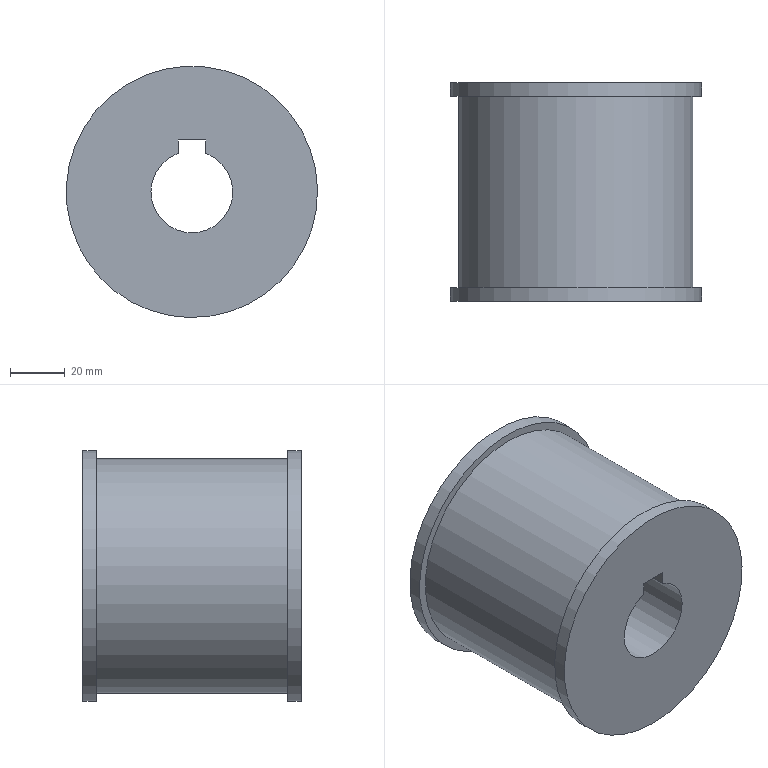Part | STEP file | SN10_001_009_POLIA | 1 solid | 11 faces | box 92 x 80 x 92 mm | volume 413118 mm3 | plane 7 | cylinder 4 | commonest cylinder face diameters 92 x2 30 x1 86 x1
STEP:
#1=CARTESIAN_POINT('',(0.,0.,0.));
#2=DIRECTION('',(0.,0.,1.));
#3=DIRECTION('',(1.,0.,0.));
#4=AXIS2_PLACEMENT_3D('',#1,#2,#3);
#5=CARTESIAN_POINT('',(6005.,-140.,19.));
#6=VERTEX_POINT('',#5);
#7=CARTESIAN_POINT('',(5995.,-140.,19.));
#8=VERTEX_POINT('',#7);
#9=CARTESIAN_POINT('',(6005.,-140.,19.));
#10=DIRECTION('',(-1.,0.,0.));
#11=VECTOR('',#10,1.);
#12=LINE('',#9,#11);
#13=CARTESIAN_POINT('',(6005.,-60.,19.));
#14=DIRECTION('',(0.,0.,1.));
#15=DIRECTION('',(1.,0.,0.));
#16=AXIS2_PLACEMENT_3D('',#13,#14,#15);
#17=PLANE('',#16);
#18=CARTESIAN_POINT('',(0.,-80.));
#19=DIRECTION('',(-1.,0.));
#20=VECTOR('',#19,1.);
#21=LINE('',#18,#20);
#22=(GEOMETRIC_REPRESENTATION_CONTEXT(2)PARAMETRIC_REPRESENTATION_CONTEXT()REPRESENTATION_CONTEXT('',''));
#23=DEFINITIONAL_REPRESENTATION('',(#21),#22);
#24=PCURVE('',#17,#23);
#25=CARTESIAN_POINT('',(6000.,-140.,0.));
#26=DIRECTION('',(0.,1.,0.));
#27=DIRECTION('',(0.,0.,1.));
#28=AXIS2_PLACEMENT_3D('',#25,#26,#27);
#29=PLANE('',#28);
#30=CARTESIAN_POINT('',(19.,5.));
#31=DIRECTION('',(0.,-1.));
#32=VECTOR('',#31,1.);
#33=LINE('',#30,#32);
#34=(GEOMETRIC_REPRESENTATION_CONTEXT(2)PARAMETRIC_REPRESENTATION_CONTEXT()REPRESENTATION_CONTEXT('',''));
#35=DEFINITIONAL_REPRESENTATION('',(#33),#34);
#36=PCURVE('',#29,#35);
#37=SURFACE_CURVE('',#12,(#24,#36),.PCURVE_S1.);
#38=EDGE_CURVE('',#6,#8,#37,.T.);
#39=ORIENTED_EDGE('',*,*,#38,.T.);
#40=CARTESIAN_POINT('',(5995.,-60.,19.));
#41=VERTEX_POINT('',#40);
#42=CARTESIAN_POINT('',(5995.,-60.,19.));
#43=DIRECTION('',(0.,-1.,0.));
#44=VECTOR('',#43,1.);
#45=LINE('',#42,#44);
#46=CARTESIAN_POINT('',(-10.,0.));
#47=DIRECTION('',(0.,-1.));
#48=VECTOR('',#47,1.);
#49=LINE('',#46,#48);
#50=(GEOMETRIC_REPRESENTATION_CONTEXT(2)PARAMETRIC_REPRESENTATION_CONTEXT()REPRESENTATION_CONTEXT('',''));
#51=DEFINITIONAL_REPRESENTATION('',(#49),#50);
#52=PCURVE('',#17,#51);
#53=CARTESIAN_POINT('',(5995.,-60.,11.));
#54=DIRECTION('',(1.,0.,0.));
#55=DIRECTION('',(0.,0.,-1.));
#56=AXIS2_PLACEMENT_3D('',#53,#54,#55);
#57=PLANE('',#56);
#58=CARTESIAN_POINT('',(-8.,0.));
#59=DIRECTION('',(0.,-1.));
#60=VECTOR('',#59,1.);
#61=LINE('',#58,#60);
#62=(GEOMETRIC_REPRESENTATION_CONTEXT(2)PARAMETRIC_REPRESENTATION_CONTEXT()REPRESENTATION_CONTEXT('',''));
#63=DEFINITIONAL_REPRESENTATION('',(#61),#62);
#64=PCURVE('',#57,#63);
#65=SURFACE_CURVE('',#45,(#52,#64),.PCURVE_S1.);
#66=EDGE_CURVE('',#41,#8,#65,.T.);
#67=ORIENTED_EDGE('',*,*,#66,.F.);
#68=CARTESIAN_POINT('',(6005.,-60.,19.));
#69=VERTEX_POINT('',#68);
#70=CARTESIAN_POINT('',(6005.,-60.,19.));
#71=DIRECTION('',(-1.,0.,0.));
#72=VECTOR('',#71,1.);
#73=LINE('',#70,#72);
#74=CARTESIAN_POINT('',(0.,0.));
#75=DIRECTION('',(-1.,0.));
#76=VECTOR('',#75,1.);
#77=LINE('',#74,#76);
#78=(GEOMETRIC_REPRESENTATION_CONTEXT(2)PARAMETRIC_REPRESENTATION_CONTEXT()REPRESENTATION_CONTEXT('',''));
#79=DEFINITIONAL_REPRESENTATION('',(#77),#78);
#80=PCURVE('',#17,#79);
#81=CARTESIAN_POINT('',(6000.,-60.,46.));
#82=DIRECTION('',(0.,1.,0.));
#83=DIRECTION('',(0.,0.,1.));
#84=AXIS2_PLACEMENT_3D('',#81,#82,#83);
#85=PLANE('',#84);
#86=CARTESIAN_POINT('',(-27.,5.));
#87=DIRECTION('',(0.,-1.));
#88=VECTOR('',#87,1.);
#89=LINE('',#86,#88);
#90=(GEOMETRIC_REPRESENTATION_CONTEXT(2)PARAMETRIC_REPRESENTATION_CONTEXT()REPRESENTATION_CONTEXT('',''));
#91=DEFINITIONAL_REPRESENTATION('',(#89),#90);
#92=PCURVE('',#85,#91);
#93=SURFACE_CURVE('',#73,(#80,#92),.PCURVE_S1.);
#94=EDGE_CURVE('',#69,#41,#93,.T.);
#95=ORIENTED_EDGE('',*,*,#94,.F.);
#96=CARTESIAN_POINT('',(6005.,-60.,19.));
#97=DIRECTION('',(0.,-1.,0.));
#98=VECTOR('',#97,1.);
#99=LINE('',#96,#98);
#100=CARTESIAN_POINT('',(0.,0.));
#101=DIRECTION('',(0.,-1.));
#102=VECTOR('',#101,1.);
#103=LINE('',#100,#102);
#104=(GEOMETRIC_REPRESENTATION_CONTEXT(2)PARAMETRIC_REPRESENTATION_CONTEXT()REPRESENTATION_CONTEXT('',''));
#105=DEFINITIONAL_REPRESENTATION('',(#103),#104);
#106=PCURVE('',#17,#105);
#107=CARTESIAN_POINT('',(6005.,-60.,19.));
#108=DIRECTION('',(-1.,0.,0.));
#109=DIRECTION('',(0.,0.,1.));
#110=AXIS2_PLACEMENT_3D('',#107,#108,#109);
#111=PLANE('',#110);
#112=CARTESIAN_POINT('',(0.,0.));
#113=DIRECTION('',(0.,-1.));
#114=VECTOR('',#113,1.);
#115=LINE('',#112,#114);
#116=(GEOMETRIC_REPRESENTATION_CONTEXT(2)PARAMETRIC_REPRESENTATION_CONTEXT()REPRESENTATION_CONTEXT('',''));
#117=DEFINITIONAL_REPRESENTATION('',(#115),#116);
#118=PCURVE('',#111,#117);
#119=SURFACE_CURVE('',#99,(#106,#118),.PCURVE_S1.);
#120=EDGE_CURVE('',#69,#6,#119,.T.);
#121=ORIENTED_EDGE('',*,*,#120,.T.);
#122=EDGE_LOOP('',(#39,#67,#95,#121));
#123=FACE_BOUND('',#122,.T.);
#124=ADVANCED_FACE('',(#123),#17,.F.);
#125=ORIENTED_EDGE('',*,*,#120,.F.);
#126=CARTESIAN_POINT('',(6005.,-60.,14.142));
#127=VERTEX_POINT('',#126);
#128=CARTESIAN_POINT('',(6005.,-60.,19.));
#129=DIRECTION('',(0.,0.,-1.));
#130=VECTOR('',#129,1.);
#131=LINE('',#128,#130);
#132=CARTESIAN_POINT('',(0.,0.));
#133=DIRECTION('',(-1.,0.));
#134=VECTOR('',#133,1.);
#135=LINE('',#132,#134);
#136=(GEOMETRIC_REPRESENTATION_CONTEXT(2)PARAMETRIC_REPRESENTATION_CONTEXT()REPRESENTATION_CONTEXT('',''));
#137=DEFINITIONAL_REPRESENTATION('',(#135),#136);
#138=PCURVE('',#111,#137);
#139=CARTESIAN_POINT('',(-27.,5.));
#140=DIRECTION('',(-1.,0.));
#141=VECTOR('',#140,1.);
#142=LINE('',#139,#141);
#143=(GEOMETRIC_REPRESENTATION_CONTEXT(2)PARAMETRIC_REPRESENTATION_CONTEXT()REPRESENTATION_CONTEXT('',''));
#144=DEFINITIONAL_REPRESENTATION('',(#142),#143);
#145=PCURVE('',#85,#144);
#146=SURFACE_CURVE('',#131,(#138,#145),.PCURVE_S1.);
#147=EDGE_CURVE('',#69,#127,#146,.T.);
#148=ORIENTED_EDGE('',*,*,#147,.T.);
#149=CARTESIAN_POINT('',(6005.,-140.,14.142));
#150=VERTEX_POINT('',#149);
#151=CARTESIAN_POINT('',(6005.,-60.,14.142));
#152=DIRECTION('',(0.,-1.,0.));
#153=VECTOR('',#152,1.);
#154=LINE('',#151,#153);
#155=CARTESIAN_POINT('',(-4.858,0.));
#156=DIRECTION('',(0.,-1.));
#157=VECTOR('',#156,1.);
#158=LINE('',#155,#157);
#159=(GEOMETRIC_REPRESENTATION_CONTEXT(2)PARAMETRIC_REPRESENTATION_CONTEXT()REPRESENTATION_CONTEXT('',''));
#160=DEFINITIONAL_REPRESENTATION('',(#158),#159);
#161=PCURVE('',#111,#160);
#162=CARTESIAN_POINT('',(6000.,-60.1,0.));
#163=DIRECTION('',(0.,-1.,0.));
#164=DIRECTION('',(0.8776,0.,0.4794));
#165=AXIS2_PLACEMENT_3D('',#162,#163,#164);
#166=CYLINDRICAL_SURFACE('',#165,15.);
#167=CARTESIAN_POINT('',(7.014,-0.1));
#168=DIRECTION('',(0.,1.));
#169=VECTOR('',#168,1.);
#170=LINE('',#167,#169);
#171=(GEOMETRIC_REPRESENTATION_CONTEXT(2)PARAMETRIC_REPRESENTATION_CONTEXT()REPRESENTATION_CONTEXT('',''));
#172=DEFINITIONAL_REPRESENTATION('',(#170),#171);
#173=PCURVE('',#166,#172);
#174=SURFACE_CURVE('',#154,(#161,#173),.PCURVE_S1.);
#175=EDGE_CURVE('',#127,#150,#174,.T.);
#176=ORIENTED_EDGE('',*,*,#175,.T.);
#177=CARTESIAN_POINT('',(6005.,-140.,19.));
#178=DIRECTION('',(0.,0.,-1.));
#179=VECTOR('',#178,1.);
#180=LINE('',#177,#179);
#181=CARTESIAN_POINT('',(0.,-80.));
#182=DIRECTION('',(-1.,0.));
#183=VECTOR('',#182,1.);
#184=LINE('',#181,#183);
#185=(GEOMETRIC_REPRESENTATION_CONTEXT(2)PARAMETRIC_REPRESENTATION_CONTEXT()REPRESENTATION_CONTEXT('',''));
#186=DEFINITIONAL_REPRESENTATION('',(#184),#185);
#187=PCURVE('',#111,#186);
#188=CARTESIAN_POINT('',(19.,5.));
#189=DIRECTION('',(-1.,0.));
#190=VECTOR('',#189,1.);
#191=LINE('',#188,#190);
#192=(GEOMETRIC_REPRESENTATION_CONTEXT(2)PARAMETRIC_REPRESENTATION_CONTEXT()REPRESENTATION_CONTEXT('',''));
#193=DEFINITIONAL_REPRESENTATION('',(#191),#192);
#194=PCURVE('',#29,#193);
#195=SURFACE_CURVE('',#180,(#187,#194),.PCURVE_S1.);
#196=EDGE_CURVE('',#6,#150,#195,.T.);
#197=ORIENTED_EDGE('',*,*,#196,.F.);
#198=EDGE_LOOP('',(#125,#148,#176,#197));
#199=FACE_BOUND('',#198,.T.);
#200=ADVANCED_FACE('',(#199),#111,.T.);
#201=CARTESIAN_POINT('',(5977.946,-60.,-40.369));
#202=VERTEX_POINT('',#201);
#203=CARTESIAN_POINT('',(6000.,-60.,0.));
#204=DIRECTION('',(0.,1.,0.));
#205=DIRECTION('',(1.,0.,0.));
#206=AXIS2_PLACEMENT_3D('',#203,#204,#205);
#207=CIRCLE('',#206,46.);
#208=CARTESIAN_POINT('',(-46.,0.));
#209=DIRECTION('',(0.,1.));
#210=AXIS2_PLACEMENT_2D('',#208,#209);
#211=CIRCLE('',#210,46.);
#212=(GEOMETRIC_REPRESENTATION_CONTEXT(2)PARAMETRIC_REPRESENTATION_CONTEXT()REPRESENTATION_CONTEXT('',''));
#213=DEFINITIONAL_REPRESENTATION('',(#211),#212);
#214=PCURVE('',#85,#213);
#215=CARTESIAN_POINT('',(6000.,-100.,0.));
#216=DIRECTION('',(0.,1.,0.));
#217=DIRECTION('',(0.4794,0.,0.8776));
#218=AXIS2_PLACEMENT_3D('',#215,#216,#217);
#219=CYLINDRICAL_SURFACE('',#218,46.);
#220=CARTESIAN_POINT('',(1.071,40.));
#221=DIRECTION('',(1.,0.));
#222=VECTOR('',#221,1.);
#223=LINE('',#220,#222);
#224=(GEOMETRIC_REPRESENTATION_CONTEXT(2)PARAMETRIC_REPRESENTATION_CONTEXT()REPRESENTATION_CONTEXT('',''));
#225=DEFINITIONAL_REPRESENTATION('',(#223),#224);
#226=PCURVE('',#219,#225);
#227=SURFACE_CURVE('',#207,(#214,#226),.PCURVE_S1.);
#228=EDGE_CURVE('',#202,#202,#227,.T.);
#229=ORIENTED_EDGE('',*,*,#228,.T.);
#230=EDGE_LOOP('',(#229));
#231=FACE_BOUND('',#230,.T.);
#232=CARTESIAN_POINT('',(5995.,-60.,14.142));
#233=VERTEX_POINT('',#232);
#234=CARTESIAN_POINT('',(6000.,-60.,0.));
#235=DIRECTION('',(0.,1.,0.));
#236=DIRECTION('',(1.,0.,0.));
#237=AXIS2_PLACEMENT_3D('',#234,#235,#236);
#238=CIRCLE('',#237,15.);
#239=CARTESIAN_POINT('',(-46.,0.));
#240=DIRECTION('',(0.,1.));
#241=AXIS2_PLACEMENT_2D('',#239,#240);
#242=CIRCLE('',#241,15.);
#243=(GEOMETRIC_REPRESENTATION_CONTEXT(2)PARAMETRIC_REPRESENTATION_CONTEXT()REPRESENTATION_CONTEXT('',''));
#244=DEFINITIONAL_REPRESENTATION('',(#242),#243);
#245=PCURVE('',#85,#244);
#246=CARTESIAN_POINT('',(12.066,-0.1));
#247=DIRECTION('',(-1.,0.));
#248=VECTOR('',#247,1.);
#249=LINE('',#246,#248);
#250=(GEOMETRIC_REPRESENTATION_CONTEXT(2)PARAMETRIC_REPRESENTATION_CONTEXT()REPRESENTATION_CONTEXT('',''));
#251=DEFINITIONAL_REPRESENTATION('',(#249),#250);
#252=PCURVE('',#166,#251);
#253=SURFACE_CURVE('',#238,(#245,#252),.PCURVE_S1.);
#254=EDGE_CURVE('',#127,#233,#253,.T.);
#255=ORIENTED_EDGE('',*,*,#254,.F.);
#256=ORIENTED_EDGE('',*,*,#147,.F.);
#257=ORIENTED_EDGE('',*,*,#94,.T.);
#258=CARTESIAN_POINT('',(5995.,-60.,14.142));
#259=DIRECTION('',(0.,0.,1.));
#260=VECTOR('',#259,1.);
#261=LINE('',#258,#260);
#262=CARTESIAN_POINT('',(-31.858,-5.));
#263=DIRECTION('',(1.,0.));
#264=VECTOR('',#263,1.);
#265=LINE('',#262,#264);
#266=(GEOMETRIC_REPRESENTATION_CONTEXT(2)PARAMETRIC_REPRESENTATION_CONTEXT()REPRESENTATION_CONTEXT('',''));
#267=DEFINITIONAL_REPRESENTATION('',(#265),#266);
#268=PCURVE('',#85,#267);
#269=CARTESIAN_POINT('',(-3.142,0.));
#270=DIRECTION('',(-1.,0.));
#271=VECTOR('',#270,1.);
#272=LINE('',#269,#271);
#273=(GEOMETRIC_REPRESENTATION_CONTEXT(2)PARAMETRIC_REPRESENTATION_CONTEXT()REPRESENTATION_CONTEXT('',''));
#274=DEFINITIONAL_REPRESENTATION('',(#272),#273);
#275=PCURVE('',#57,#274);
#276=SURFACE_CURVE('',#261,(#268,#275),.PCURVE_S1.);
#277=EDGE_CURVE('',#233,#41,#276,.T.);
#278=ORIENTED_EDGE('',*,*,#277,.F.);
#279=EDGE_LOOP('',(#255,#256,#257,#278));
#280=FACE_BOUND('',#279,.T.);
#281=ADVANCED_FACE('',(#231,#280),#85,.T.);
#282=CARTESIAN_POINT('',(5977.946,-140.,-40.369));
#283=VERTEX_POINT('',#282);
#284=CARTESIAN_POINT('',(6000.,-140.,0.));
#285=DIRECTION('',(0.,1.,0.));
#286=DIRECTION('',(1.,0.,0.));
#287=AXIS2_PLACEMENT_3D('',#284,#285,#286);
#288=CIRCLE('',#287,46.);
#289=CARTESIAN_POINT('',(0.,0.));
#290=DIRECTION('',(0.,1.));
#291=AXIS2_PLACEMENT_2D('',#289,#290);
#292=CIRCLE('',#291,46.);
#293=(GEOMETRIC_REPRESENTATION_CONTEXT(2)PARAMETRIC_REPRESENTATION_CONTEXT()REPRESENTATION_CONTEXT('',''));
#294=DEFINITIONAL_REPRESENTATION('',(#292),#293);
#295=PCURVE('',#29,#294);
#296=CARTESIAN_POINT('',(6000.,-100.,0.));
#297=DIRECTION('',(0.,1.,0.));
#298=DIRECTION('',(0.4794,0.,0.8776));
#299=AXIS2_PLACEMENT_3D('',#296,#297,#298);
#300=CYLINDRICAL_SURFACE('',#299,46.);
#301=CARTESIAN_POINT('',(1.071,-40.));
#302=DIRECTION('',(1.,0.));
#303=VECTOR('',#302,1.);
#304=LINE('',#301,#303);
#305=(GEOMETRIC_REPRESENTATION_CONTEXT(2)PARAMETRIC_REPRESENTATION_CONTEXT()REPRESENTATION_CONTEXT('',''));
#306=DEFINITIONAL_REPRESENTATION('',(#304),#305);
#307=PCURVE('',#300,#306);
#308=SURFACE_CURVE('',#288,(#295,#307),.PCURVE_S1.);
#309=EDGE_CURVE('',#283,#283,#308,.T.);
#310=ORIENTED_EDGE('',*,*,#309,.F.);
#311=EDGE_LOOP('',(#310));
#312=FACE_BOUND('',#311,.T.);
#313=CARTESIAN_POINT('',(5995.,-140.,14.142));
#314=VERTEX_POINT('',#313);
#315=CARTESIAN_POINT('',(5995.,-140.,14.142));
#316=DIRECTION('',(0.,0.,1.));
#317=VECTOR('',#316,1.);
#318=LINE('',#315,#317);
#319=CARTESIAN_POINT('',(14.142,-5.));
#320=DIRECTION('',(1.,0.));
#321=VECTOR('',#320,1.);
#322=LINE('',#319,#321);
#323=(GEOMETRIC_REPRESENTATION_CONTEXT(2)PARAMETRIC_REPRESENTATION_CONTEXT()REPRESENTATION_CONTEXT('',''));
#324=DEFINITIONAL_REPRESENTATION('',(#322),#323);
#325=PCURVE('',#29,#324);
#326=CARTESIAN_POINT('',(-3.142,-80.));
#327=DIRECTION('',(-1.,0.));
#328=VECTOR('',#327,1.);
#329=LINE('',#326,#328);
#330=(GEOMETRIC_REPRESENTATION_CONTEXT(2)PARAMETRIC_REPRESENTATION_CONTEXT()REPRESENTATION_CONTEXT('',''));
#331=DEFINITIONAL_REPRESENTATION('',(#329),#330);
#332=PCURVE('',#57,#331);
#333=SURFACE_CURVE('',#318,(#325,#332),.PCURVE_S1.);
#334=EDGE_CURVE('',#314,#8,#333,.T.);
#335=ORIENTED_EDGE('',*,*,#334,.T.);
#336=ORIENTED_EDGE('',*,*,#38,.F.);
#337=ORIENTED_EDGE('',*,*,#196,.T.);
#338=CARTESIAN_POINT('',(6000.,-140.,0.));
#339=DIRECTION('',(0.,1.,0.));
#340=DIRECTION('',(1.,0.,0.));
#341=AXIS2_PLACEMENT_3D('',#338,#339,#340);
#342=CIRCLE('',#341,15.);
#343=CARTESIAN_POINT('',(0.,0.));
#344=DIRECTION('',(0.,1.));
#345=AXIS2_PLACEMENT_2D('',#343,#344);
#346=CIRCLE('',#345,15.);
#347=(GEOMETRIC_REPRESENTATION_CONTEXT(2)PARAMETRIC_REPRESENTATION_CONTEXT()REPRESENTATION_CONTEXT('',''));
#348=DEFINITIONAL_REPRESENTATION('',(#346),#347);
#349=PCURVE('',#29,#348);
#350=CARTESIAN_POINT('',(12.066,79.9));
#351=DIRECTION('',(-1.,0.));
#352=VECTOR('',#351,1.);
#353=LINE('',#350,#352);
#354=(GEOMETRIC_REPRESENTATION_CONTEXT(2)PARAMETRIC_REPRESENTATION_CONTEXT()REPRESENTATION_CONTEXT('',''));
#355=DEFINITIONAL_REPRESENTATION('',(#353),#354);
#356=PCURVE('',#166,#355);
#357=SURFACE_CURVE('',#342,(#349,#356),.PCURVE_S1.);
#358=EDGE_CURVE('',#150,#314,#357,.T.);
#359=ORIENTED_EDGE('',*,*,#358,.T.);
#360=EDGE_LOOP('',(#335,#336,#337,#359));
#361=FACE_BOUND('',#360,.T.);
#362=ADVANCED_FACE('',(#312,#361),#29,.F.);
#363=ORIENTED_EDGE('',*,*,#358,.T.);
#364=CARTESIAN_POINT('',(5995.,-60.,14.142));
#365=DIRECTION('',(0.,-1.,0.));
#366=VECTOR('',#365,1.);
#367=LINE('',#364,#366);
#368=CARTESIAN_POINT('',(1.411,-0.1));
#369=DIRECTION('',(0.,1.));
#370=VECTOR('',#369,1.);
#371=LINE('',#368,#370);
#372=(GEOMETRIC_REPRESENTATION_CONTEXT(2)PARAMETRIC_REPRESENTATION_CONTEXT()REPRESENTATION_CONTEXT('',''));
#373=DEFINITIONAL_REPRESENTATION('',(#371),#372);
#374=PCURVE('',#166,#373);
#375=CARTESIAN_POINT('',(-3.142,0.));
#376=DIRECTION('',(0.,-1.));
#377=VECTOR('',#376,1.);
#378=LINE('',#375,#377);
#379=(GEOMETRIC_REPRESENTATION_CONTEXT(2)PARAMETRIC_REPRESENTATION_CONTEXT()REPRESENTATION_CONTEXT('',''));
#380=DEFINITIONAL_REPRESENTATION('',(#378),#379);
#381=PCURVE('',#57,#380);
#382=SURFACE_CURVE('',#367,(#374,#381),.PCURVE_S1.);
#383=EDGE_CURVE('',#233,#314,#382,.T.);
#384=ORIENTED_EDGE('',*,*,#383,.F.);
#385=ORIENTED_EDGE('',*,*,#254,.F.);
#386=ORIENTED_EDGE('',*,*,#175,.T.);
#387=EDGE_LOOP('',(#363,#384,#385,#386));
#388=FACE_BOUND('',#387,.F.);
#389=ADVANCED_FACE('',(#388),#166,.F.);
#390=ORIENTED_EDGE('',*,*,#228,.F.);
#391=CARTESIAN_POINT('',(5977.946,-65.,-40.369));
#392=VERTEX_POINT('',#391);
#393=CARTESIAN_POINT('',(5977.946,-65.,-40.369));
#394=CARTESIAN_POINT('',(5977.946,-60.,-40.369));
#395=B_SPLINE_CURVE_WITH_KNOTS('',1,(#393,#394),.UNSPECIFIED.,.F.,.F.,(2,2),(35.,40.),.PIECEWISE_BEZIER_KNOTS.);
#396=CARTESIAN_POINT('',(3.142,0.));
#397=DIRECTION('',(0.,1.));
#398=VECTOR('',#397,1.);
#399=LINE('',#396,#398);
#400=(GEOMETRIC_REPRESENTATION_CONTEXT(2)PARAMETRIC_REPRESENTATION_CONTEXT()REPRESENTATION_CONTEXT('',''));
#401=DEFINITIONAL_REPRESENTATION('',(#399),#400);
#402=PCURVE('',#219,#401);
#403=CARTESIAN_POINT('',(9.425,0.));
#404=DIRECTION('',(0.,1.));
#405=VECTOR('',#404,1.);
#406=LINE('',#403,#405);
#407=(GEOMETRIC_REPRESENTATION_CONTEXT(2)PARAMETRIC_REPRESENTATION_CONTEXT()REPRESENTATION_CONTEXT('',''));
#408=DEFINITIONAL_REPRESENTATION('',(#406),#407);
#409=PCURVE('',#219,#408);
#410=SEAM_CURVE('',#395,(#402,#409),.PCURVE_S1.);
#411=EDGE_CURVE('',#392,#202,#410,.T.);
#412=ORIENTED_EDGE('',*,*,#411,.F.);
#413=CARTESIAN_POINT('',(6000.,-65.,0.));
#414=DIRECTION('',(0.,1.,0.));
#415=DIRECTION('',(1.,0.,0.));
#416=AXIS2_PLACEMENT_3D('',#413,#414,#415);
#417=CIRCLE('',#416,46.);
#418=CARTESIAN_POINT('',(1.071,35.));
#419=DIRECTION('',(1.,0.));
#420=VECTOR('',#419,1.);
#421=LINE('',#418,#420);
#422=(GEOMETRIC_REPRESENTATION_CONTEXT(2)PARAMETRIC_REPRESENTATION_CONTEXT()REPRESENTATION_CONTEXT('',''));
#423=DEFINITIONAL_REPRESENTATION('',(#421),#422);
#424=PCURVE('',#219,#423);
#425=CARTESIAN_POINT('',(6000.,-65.,43.));
#426=DIRECTION('',(0.,1.,0.));
#427=DIRECTION('',(0.,0.,1.));
#428=AXIS2_PLACEMENT_3D('',#425,#426,#427);
#429=PLANE('',#428);
#430=CARTESIAN_POINT('',(-43.,0.));
#431=DIRECTION('',(0.,1.));
#432=AXIS2_PLACEMENT_2D('',#430,#431);
#433=CIRCLE('',#432,46.);
#434=(GEOMETRIC_REPRESENTATION_CONTEXT(2)PARAMETRIC_REPRESENTATION_CONTEXT()REPRESENTATION_CONTEXT('',''));
#435=DEFINITIONAL_REPRESENTATION('',(#433),#434);
#436=PCURVE('',#429,#435);
#437=SURFACE_CURVE('',#417,(#424,#436),.PCURVE_S1.);
#438=EDGE_CURVE('',#392,#392,#437,.T.);
#439=ORIENTED_EDGE('',*,*,#438,.T.);
#440=ORIENTED_EDGE('',*,*,#411,.T.);
#441=EDGE_LOOP('',(#390,#412,#439,#440));
#442=FACE_BOUND('',#441,.T.);
#443=ADVANCED_FACE('',(#442),#219,.T.);
#444=ORIENTED_EDGE('',*,*,#438,.F.);
#445=EDGE_LOOP('',(#444));
#446=FACE_BOUND('',#445,.T.);
#447=CARTESIAN_POINT('',(5979.385,-65.,-37.736));
#448=VERTEX_POINT('',#447);
#449=CARTESIAN_POINT('',(6000.,-65.,0.));
#450=DIRECTION('',(0.,1.,0.));
#451=DIRECTION('',(1.,0.,0.));
#452=AXIS2_PLACEMENT_3D('',#449,#450,#451);
#453=CIRCLE('',#452,43.);
#454=CARTESIAN_POINT('',(-43.,0.));
#455=DIRECTION('',(0.,1.));
#456=AXIS2_PLACEMENT_2D('',#454,#455);
#457=CIRCLE('',#456,43.);
#458=(GEOMETRIC_REPRESENTATION_CONTEXT(2)PARAMETRIC_REPRESENTATION_CONTEXT()REPRESENTATION_CONTEXT('',''));
#459=DEFINITIONAL_REPRESENTATION('',(#457),#458);
#460=PCURVE('',#429,#459);
#461=CARTESIAN_POINT('',(6000.,-100.,0.));
#462=DIRECTION('',(0.,1.,0.));
#463=DIRECTION('',(0.4794,0.,0.8776));
#464=AXIS2_PLACEMENT_3D('',#461,#462,#463);
#465=CYLINDRICAL_SURFACE('',#464,43.);
#466=CARTESIAN_POINT('',(1.071,35.));
#467=DIRECTION('',(1.,0.));
#468=VECTOR('',#467,1.);
#469=LINE('',#466,#468);
#470=(GEOMETRIC_REPRESENTATION_CONTEXT(2)PARAMETRIC_REPRESENTATION_CONTEXT()REPRESENTATION_CONTEXT('',''));
#471=DEFINITIONAL_REPRESENTATION('',(#469),#470);
#472=PCURVE('',#465,#471);
#473=SURFACE_CURVE('',#453,(#460,#472),.PCURVE_S1.);
#474=EDGE_CURVE('',#448,#448,#473,.T.);
#475=ORIENTED_EDGE('',*,*,#474,.T.);
#476=EDGE_LOOP('',(#475));
#477=FACE_BOUND('',#476,.T.);
#478=ADVANCED_FACE('',(#446,#477),#429,.F.);
#479=ORIENTED_EDGE('',*,*,#474,.F.);
#480=CARTESIAN_POINT('',(5979.385,-135.,-37.736));
#481=VERTEX_POINT('',#480);
#482=CARTESIAN_POINT('',(5979.385,-135.,-37.736));
#483=CARTESIAN_POINT('',(5979.385,-65.,-37.736));
#484=B_SPLINE_CURVE_WITH_KNOTS('',1,(#482,#483),.UNSPECIFIED.,.F.,.F.,(2,2),(-35.,35.),.PIECEWISE_BEZIER_KNOTS.);
#485=CARTESIAN_POINT('',(3.142,0.));
#486=DIRECTION('',(0.,1.));
#487=VECTOR('',#486,1.);
#488=LINE('',#485,#487);
#489=(GEOMETRIC_REPRESENTATION_CONTEXT(2)PARAMETRIC_REPRESENTATION_CONTEXT()REPRESENTATION_CONTEXT('',''));
#490=DEFINITIONAL_REPRESENTATION('',(#488),#489);
#491=PCURVE('',#465,#490);
#492=CARTESIAN_POINT('',(9.425,0.));
#493=DIRECTION('',(0.,1.));
#494=VECTOR('',#493,1.);
#495=LINE('',#492,#494);
#496=(GEOMETRIC_REPRESENTATION_CONTEXT(2)PARAMETRIC_REPRESENTATION_CONTEXT()REPRESENTATION_CONTEXT('',''));
#497=DEFINITIONAL_REPRESENTATION('',(#495),#496);
#498=PCURVE('',#465,#497);
#499=SEAM_CURVE('',#484,(#491,#498),.PCURVE_S1.);
#500=EDGE_CURVE('',#481,#448,#499,.T.);
#501=ORIENTED_EDGE('',*,*,#500,.F.);
#502=CARTESIAN_POINT('',(6000.,-135.,0.));
#503=DIRECTION('',(0.,1.,0.));
#504=DIRECTION('',(1.,0.,0.));
#505=AXIS2_PLACEMENT_3D('',#502,#503,#504);
#506=CIRCLE('',#505,43.);
#507=CARTESIAN_POINT('',(1.071,-35.));
#508=DIRECTION('',(1.,0.));
#509=VECTOR('',#508,1.);
#510=LINE('',#507,#509);
#511=(GEOMETRIC_REPRESENTATION_CONTEXT(2)PARAMETRIC_REPRESENTATION_CONTEXT()REPRESENTATION_CONTEXT('',''));
#512=DEFINITIONAL_REPRESENTATION('',(#510),#511);
#513=PCURVE('',#465,#512);
#514=CARTESIAN_POINT('',(6000.,-135.,46.));
#515=DIRECTION('',(0.,1.,0.));
#516=DIRECTION('',(0.,0.,1.));
#517=AXIS2_PLACEMENT_3D('',#514,#515,#516);
#518=PLANE('',#517);
#519=CARTESIAN_POINT('',(-46.,0.));
#520=DIRECTION('',(0.,1.));
#521=AXIS2_PLACEMENT_2D('',#519,#520);
#522=CIRCLE('',#521,43.);
#523=(GEOMETRIC_REPRESENTATION_CONTEXT(2)PARAMETRIC_REPRESENTATION_CONTEXT()REPRESENTATION_CONTEXT('',''));
#524=DEFINITIONAL_REPRESENTATION('',(#522),#523);
#525=PCURVE('',#518,#524);
#526=SURFACE_CURVE('',#506,(#513,#525),.PCURVE_S1.);
#527=EDGE_CURVE('',#481,#481,#526,.T.);
#528=ORIENTED_EDGE('',*,*,#527,.T.);
#529=ORIENTED_EDGE('',*,*,#500,.T.);
#530=EDGE_LOOP('',(#479,#501,#528,#529));
#531=FACE_BOUND('',#530,.T.);
#532=ADVANCED_FACE('',(#531),#465,.T.);
#533=CARTESIAN_POINT('',(5977.946,-135.,-40.369));
#534=VERTEX_POINT('',#533);
#535=CARTESIAN_POINT('',(6000.,-135.,0.));
#536=DIRECTION('',(0.,1.,0.));
#537=DIRECTION('',(1.,0.,0.));
#538=AXIS2_PLACEMENT_3D('',#535,#536,#537);
#539=CIRCLE('',#538,46.);
#540=CARTESIAN_POINT('',(-46.,0.));
#541=DIRECTION('',(0.,1.));
#542=AXIS2_PLACEMENT_2D('',#540,#541);
#543=CIRCLE('',#542,46.);
#544=(GEOMETRIC_REPRESENTATION_CONTEXT(2)PARAMETRIC_REPRESENTATION_CONTEXT()REPRESENTATION_CONTEXT('',''));
#545=DEFINITIONAL_REPRESENTATION('',(#543),#544);
#546=PCURVE('',#518,#545);
#547=CARTESIAN_POINT('',(1.071,-35.));
#548=DIRECTION('',(1.,0.));
#549=VECTOR('',#548,1.);
#550=LINE('',#547,#549);
#551=(GEOMETRIC_REPRESENTATION_CONTEXT(2)PARAMETRIC_REPRESENTATION_CONTEXT()REPRESENTATION_CONTEXT('',''));
#552=DEFINITIONAL_REPRESENTATION('',(#550),#551);
#553=PCURVE('',#300,#552);
#554=SURFACE_CURVE('',#539,(#546,#553),.PCURVE_S1.);
#555=EDGE_CURVE('',#534,#534,#554,.T.);
#556=ORIENTED_EDGE('',*,*,#555,.T.);
#557=EDGE_LOOP('',(#556));
#558=FACE_BOUND('',#557,.T.);
#559=ORIENTED_EDGE('',*,*,#527,.F.);
#560=EDGE_LOOP('',(#559));
#561=FACE_BOUND('',#560,.T.);
#562=ADVANCED_FACE('',(#558,#561),#518,.T.);
#563=ORIENTED_EDGE('',*,*,#555,.F.);
#564=CARTESIAN_POINT('',(5977.946,-140.,-40.369));
#565=CARTESIAN_POINT('',(5977.946,-135.,-40.369));
#566=B_SPLINE_CURVE_WITH_KNOTS('',1,(#564,#565),.UNSPECIFIED.,.F.,.F.,(2,2),(-40.,-35.),.PIECEWISE_BEZIER_KNOTS.);
#567=CARTESIAN_POINT('',(3.142,0.));
#568=DIRECTION('',(0.,1.));
#569=VECTOR('',#568,1.);
#570=LINE('',#567,#569);
#571=(GEOMETRIC_REPRESENTATION_CONTEXT(2)PARAMETRIC_REPRESENTATION_CONTEXT()REPRESENTATION_CONTEXT('',''));
#572=DEFINITIONAL_REPRESENTATION('',(#570),#571);
#573=PCURVE('',#300,#572);
#574=CARTESIAN_POINT('',(9.425,0.));
#575=DIRECTION('',(0.,1.));
#576=VECTOR('',#575,1.);
#577=LINE('',#574,#576);
#578=(GEOMETRIC_REPRESENTATION_CONTEXT(2)PARAMETRIC_REPRESENTATION_CONTEXT()REPRESENTATION_CONTEXT('',''));
#579=DEFINITIONAL_REPRESENTATION('',(#577),#578);
#580=PCURVE('',#300,#579);
#581=SEAM_CURVE('',#566,(#573,#580),.PCURVE_S1.);
#582=EDGE_CURVE('',#283,#534,#581,.T.);
#583=ORIENTED_EDGE('',*,*,#582,.F.);
#584=ORIENTED_EDGE('',*,*,#309,.T.);
#585=ORIENTED_EDGE('',*,*,#582,.T.);
#586=EDGE_LOOP('',(#563,#583,#584,#585));
#587=FACE_BOUND('',#586,.T.);
#588=ADVANCED_FACE('',(#587),#300,.T.);
#589=ORIENTED_EDGE('',*,*,#277,.T.);
#590=ORIENTED_EDGE('',*,*,#66,.T.);
#591=ORIENTED_EDGE('',*,*,#334,.F.);
#592=ORIENTED_EDGE('',*,*,#383,.F.);
#593=EDGE_LOOP('',(#589,#590,#591,#592));
#594=FACE_BOUND('',#593,.T.);
#595=ADVANCED_FACE('',(#594),#57,.T.);
#596=CLOSED_SHELL('',(#124,#200,#281,#362,#389,#443,#478,#532,#562,#588,#595));
#597=MANIFOLD_SOLID_BREP('',#596);
#598=(LENGTH_UNIT()NAMED_UNIT(*)SI_UNIT(.MILLI.,.METRE.));
#599=UNCERTAINTY_MEASURE_WITH_UNIT(LENGTH_MEASURE(0.000002),#598,'','');
#600=(NAMED_UNIT(*)PLANE_ANGLE_UNIT()SI_UNIT($,.RADIAN.));
#601=(NAMED_UNIT(*)SI_UNIT($,.STERADIAN.)SOLID_ANGLE_UNIT());
#602=(GEOMETRIC_REPRESENTATION_CONTEXT(3)GLOBAL_UNCERTAINTY_ASSIGNED_CONTEXT((#599))GLOBAL_UNIT_ASSIGNED_CONTEXT((#598,#600,#601))REPRESENTATION_CONTEXT('',''));
#603=ADVANCED_BREP_SHAPE_REPRESENTATION('',(#4,#597),#602);